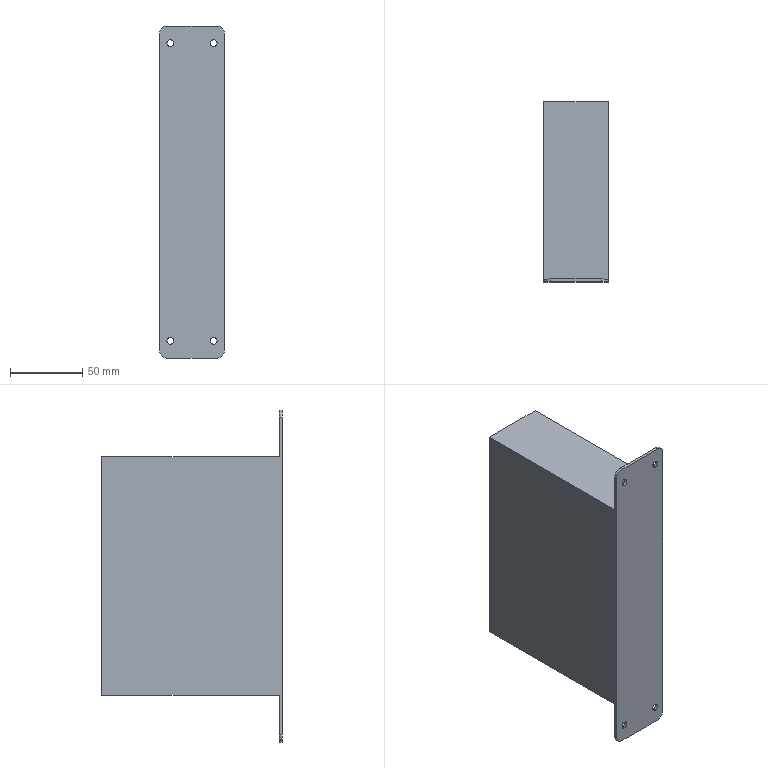Part | SolidWorks | features Extrusion 1, Fillet 1, HoleWzd 1, ICE 1 | 1 solid | 22 faces | box 45 x 125 x 230 mm | volume 933787 mm3 | cylinder 12 | plane 10 | commonest cylinder face diameters 4.8 x8 10 x4
STEP:
#1=CARTESIAN_POINT('',(-15.,0.,-105.4));
#2=VERTEX_POINT('',#1);
#3=CARTESIAN_POINT('',(-15.,0.,-100.6));
#4=VERTEX_POINT('',#3);
#5=CARTESIAN_POINT('',(-15.,0.,-103.));
#6=DIRECTION('',(0.,1.,0.));
#7=DIRECTION('',(0.,0.,1.));
#8=AXIS2_PLACEMENT_3D('',#5,#6,#7);
#9=CIRCLE('',#8,2.4);
#10=EDGE_CURVE('',#2,#4,#9,.T.);
#11=ORIENTED_EDGE('',*,*,#10,.F.);
#12=CARTESIAN_POINT('',(-15.,2.,-105.4));
#13=VERTEX_POINT('',#12);
#14=CARTESIAN_POINT('',(-15.,2.,-105.4));
#15=DIRECTION('',(0.,1.,0.));
#16=VECTOR('',#15,1000.);
#17=LINE('',#14,#16);
#18=EDGE_CURVE('',#2,#13,#17,.T.);
#19=ORIENTED_EDGE('',*,*,#18,.T.);
#20=CARTESIAN_POINT('',(-15.,2.,-100.6));
#21=VERTEX_POINT('',#20);
#22=CARTESIAN_POINT('',(-15.,2.,-103.));
#23=DIRECTION('',(0.,1.,0.));
#24=DIRECTION('',(0.,0.,1.));
#25=AXIS2_PLACEMENT_3D('',#22,#23,#24);
#26=CIRCLE('',#25,2.4);
#27=EDGE_CURVE('',#13,#21,#26,.T.);
#28=ORIENTED_EDGE('',*,*,#27,.T.);
#29=CARTESIAN_POINT('',(-15.,2.,-100.6));
#30=DIRECTION('',(0.,1.,0.));
#31=VECTOR('',#30,1000.);
#32=LINE('',#29,#31);
#33=EDGE_CURVE('',#4,#21,#32,.T.);
#34=ORIENTED_EDGE('',*,*,#33,.F.);
#35=EDGE_LOOP('',(#11,#19,#28,#34));
#36=FACE_OUTER_BOUND('',#35,.T.);
#37=CARTESIAN_POINT('',(-15.,2.,-103.));
#38=DIRECTION('',(0.,1.,0.));
#39=DIRECTION('',(0.,0.,1.));
#40=AXIS2_PLACEMENT_3D('',#37,#38,#39);
#41=CYLINDRICAL_SURFACE('',#40,2.4);
#42=ADVANCED_FACE('',(#36),#41,.F.);
#43=CARTESIAN_POINT('',(15.,0.,-105.4));
#44=VERTEX_POINT('',#43);
#45=CARTESIAN_POINT('',(15.,0.,-100.6));
#46=VERTEX_POINT('',#45);
#47=CARTESIAN_POINT('',(15.,0.,-103.));
#48=DIRECTION('',(0.,1.,0.));
#49=DIRECTION('',(0.,0.,1.));
#50=AXIS2_PLACEMENT_3D('',#47,#48,#49);
#51=CIRCLE('',#50,2.4);
#52=EDGE_CURVE('',#44,#46,#51,.T.);
#53=ORIENTED_EDGE('',*,*,#52,.F.);
#54=CARTESIAN_POINT('',(15.,2.,-105.4));
#55=VERTEX_POINT('',#54);
#56=CARTESIAN_POINT('',(15.,2.,-105.4));
#57=DIRECTION('',(0.,1.,0.));
#58=VECTOR('',#57,1000.);
#59=LINE('',#56,#58);
#60=EDGE_CURVE('',#44,#55,#59,.T.);
#61=ORIENTED_EDGE('',*,*,#60,.T.);
#62=CARTESIAN_POINT('',(15.,2.,-100.6));
#63=VERTEX_POINT('',#62);
#64=CARTESIAN_POINT('',(15.,2.,-103.));
#65=DIRECTION('',(0.,1.,0.));
#66=DIRECTION('',(0.,0.,1.));
#67=AXIS2_PLACEMENT_3D('',#64,#65,#66);
#68=CIRCLE('',#67,2.4);
#69=EDGE_CURVE('',#55,#63,#68,.T.);
#70=ORIENTED_EDGE('',*,*,#69,.T.);
#71=CARTESIAN_POINT('',(15.,2.,-100.6));
#72=DIRECTION('',(0.,1.,0.));
#73=VECTOR('',#72,1000.);
#74=LINE('',#71,#73);
#75=EDGE_CURVE('',#46,#63,#74,.T.);
#76=ORIENTED_EDGE('',*,*,#75,.F.);
#77=EDGE_LOOP('',(#53,#61,#70,#76));
#78=FACE_OUTER_BOUND('',#77,.T.);
#79=CARTESIAN_POINT('',(15.,2.,-103.));
#80=DIRECTION('',(0.,1.,0.));
#81=DIRECTION('',(0.,0.,1.));
#82=AXIS2_PLACEMENT_3D('',#79,#80,#81);
#83=CYLINDRICAL_SURFACE('',#82,2.4);
#84=ADVANCED_FACE('',(#78),#83,.F.);
#85=CARTESIAN_POINT('',(15.,0.,100.6));
#86=VERTEX_POINT('',#85);
#87=CARTESIAN_POINT('',(15.,0.,105.4));
#88=VERTEX_POINT('',#87);
#89=CARTESIAN_POINT('',(15.,0.,103.));
#90=DIRECTION('',(0.,1.,0.));
#91=DIRECTION('',(0.,0.,1.));
#92=AXIS2_PLACEMENT_3D('',#89,#90,#91);
#93=CIRCLE('',#92,2.4);
#94=EDGE_CURVE('',#86,#88,#93,.T.);
#95=ORIENTED_EDGE('',*,*,#94,.F.);
#96=CARTESIAN_POINT('',(15.,2.,100.6));
#97=VERTEX_POINT('',#96);
#98=CARTESIAN_POINT('',(15.,2.,100.6));
#99=DIRECTION('',(0.,1.,0.));
#100=VECTOR('',#99,1000.);
#101=LINE('',#98,#100);
#102=EDGE_CURVE('',#86,#97,#101,.T.);
#103=ORIENTED_EDGE('',*,*,#102,.T.);
#104=CARTESIAN_POINT('',(15.,2.,105.4));
#105=VERTEX_POINT('',#104);
#106=CARTESIAN_POINT('',(15.,2.,103.));
#107=DIRECTION('',(0.,1.,0.));
#108=DIRECTION('',(0.,0.,1.));
#109=AXIS2_PLACEMENT_3D('',#106,#107,#108);
#110=CIRCLE('',#109,2.4);
#111=EDGE_CURVE('',#97,#105,#110,.T.);
#112=ORIENTED_EDGE('',*,*,#111,.T.);
#113=CARTESIAN_POINT('',(15.,2.,105.4));
#114=DIRECTION('',(0.,1.,0.));
#115=VECTOR('',#114,1000.);
#116=LINE('',#113,#115);
#117=EDGE_CURVE('',#88,#105,#116,.T.);
#118=ORIENTED_EDGE('',*,*,#117,.F.);
#119=EDGE_LOOP('',(#95,#103,#112,#118));
#120=FACE_OUTER_BOUND('',#119,.T.);
#121=CARTESIAN_POINT('',(15.,2.,103.));
#122=DIRECTION('',(0.,1.,0.));
#123=DIRECTION('',(0.,0.,1.));
#124=AXIS2_PLACEMENT_3D('',#121,#122,#123);
#125=CYLINDRICAL_SURFACE('',#124,2.4);
#126=ADVANCED_FACE('',(#120),#125,.F.);
#127=CARTESIAN_POINT('',(-15.,0.,100.6));
#128=VERTEX_POINT('',#127);
#129=CARTESIAN_POINT('',(-15.,0.,105.4));
#130=VERTEX_POINT('',#129);
#131=CARTESIAN_POINT('',(-15.,0.,103.));
#132=DIRECTION('',(0.,1.,0.));
#133=DIRECTION('',(0.,0.,1.));
#134=AXIS2_PLACEMENT_3D('',#131,#132,#133);
#135=CIRCLE('',#134,2.4);
#136=EDGE_CURVE('',#128,#130,#135,.T.);
#137=ORIENTED_EDGE('',*,*,#136,.F.);
#138=CARTESIAN_POINT('',(-15.,2.,100.6));
#139=VERTEX_POINT('',#138);
#140=CARTESIAN_POINT('',(-15.,2.,100.6));
#141=DIRECTION('',(0.,1.,0.));
#142=VECTOR('',#141,1000.);
#143=LINE('',#140,#142);
#144=EDGE_CURVE('',#128,#139,#143,.T.);
#145=ORIENTED_EDGE('',*,*,#144,.T.);
#146=CARTESIAN_POINT('',(-15.,2.,105.4));
#147=VERTEX_POINT('',#146);
#148=CARTESIAN_POINT('',(-15.,2.,103.));
#149=DIRECTION('',(0.,1.,0.));
#150=DIRECTION('',(0.,0.,1.));
#151=AXIS2_PLACEMENT_3D('',#148,#149,#150);
#152=CIRCLE('',#151,2.4);
#153=EDGE_CURVE('',#139,#147,#152,.T.);
#154=ORIENTED_EDGE('',*,*,#153,.T.);
#155=CARTESIAN_POINT('',(-15.,2.,105.4));
#156=DIRECTION('',(0.,1.,0.));
#157=VECTOR('',#156,1000.);
#158=LINE('',#155,#157);
#159=EDGE_CURVE('',#130,#147,#158,.T.);
#160=ORIENTED_EDGE('',*,*,#159,.F.);
#161=EDGE_LOOP('',(#137,#145,#154,#160));
#162=FACE_OUTER_BOUND('',#161,.T.);
#163=CARTESIAN_POINT('',(-15.,2.,103.));
#164=DIRECTION('',(0.,1.,0.));
#165=DIRECTION('',(0.,0.,1.));
#166=AXIS2_PLACEMENT_3D('',#163,#164,#165);
#167=CYLINDRICAL_SURFACE('',#166,2.4);
#168=ADVANCED_FACE('',(#162),#167,.F.);
#169=CARTESIAN_POINT('',(22.5,2.,82.5));
#170=VERTEX_POINT('',#169);
#171=CARTESIAN_POINT('',(-22.5,2.,82.5));
#172=VERTEX_POINT('',#171);
#173=CARTESIAN_POINT('',(-22.5,2.,82.5));
#174=DIRECTION('',(-1.,0.,0.));
#175=VECTOR('',#174,1000.);
#176=LINE('',#173,#175);
#177=EDGE_CURVE('',#170,#172,#176,.T.);
#178=ORIENTED_EDGE('',*,*,#177,.F.);
#179=CARTESIAN_POINT('',(22.5,125.,82.5));
#180=VERTEX_POINT('',#179);
#181=CARTESIAN_POINT('',(22.5,125.,82.5));
#182=DIRECTION('',(0.,-1.,0.));
#183=VECTOR('',#182,1000.);
#184=LINE('',#181,#183);
#185=EDGE_CURVE('',#180,#170,#184,.T.);
#186=ORIENTED_EDGE('',*,*,#185,.F.);
#187=CARTESIAN_POINT('',(-22.5,125.,82.5));
#188=VERTEX_POINT('',#187);
#189=CARTESIAN_POINT('',(-22.5,125.,82.5));
#190=DIRECTION('',(1.,0.,0.));
#191=VECTOR('',#190,1000.);
#192=LINE('',#189,#191);
#193=EDGE_CURVE('',#188,#180,#192,.T.);
#194=ORIENTED_EDGE('',*,*,#193,.F.);
#195=CARTESIAN_POINT('',(-22.5,125.,82.5));
#196=DIRECTION('',(0.,-1.,0.));
#197=VECTOR('',#196,1000.);
#198=LINE('',#195,#197);
#199=EDGE_CURVE('',#188,#172,#198,.T.);
#200=ORIENTED_EDGE('',*,*,#199,.T.);
#201=EDGE_LOOP('',(#178,#186,#194,#200));
#202=FACE_OUTER_BOUND('',#201,.T.);
#203=CARTESIAN_POINT('',(-22.5,125.,82.5));
#204=DIRECTION('',(0.,0.,-1.));
#205=DIRECTION('',(-1.,0.,0.));
#206=AXIS2_PLACEMENT_3D('',#203,#204,#205);
#207=PLANE('',#206);
#208=ADVANCED_FACE('',(#202),#207,.F.);
#209=CARTESIAN_POINT('',(-22.5,2.,-82.5));
#210=VERTEX_POINT('',#209);
#211=CARTESIAN_POINT('',(22.5,2.,-82.5));
#212=VERTEX_POINT('',#211);
#213=CARTESIAN_POINT('',(-22.5,2.,-82.5));
#214=DIRECTION('',(1.,0.,0.));
#215=VECTOR('',#214,1000.);
#216=LINE('',#213,#215);
#217=EDGE_CURVE('',#210,#212,#216,.T.);
#218=ORIENTED_EDGE('',*,*,#217,.F.);
#219=CARTESIAN_POINT('',(-22.5,125.,-82.5));
#220=VERTEX_POINT('',#219);
#221=CARTESIAN_POINT('',(-22.5,125.,-82.5));
#222=DIRECTION('',(0.,-1.,0.));
#223=VECTOR('',#222,1000.);
#224=LINE('',#221,#223);
#225=EDGE_CURVE('',#220,#210,#224,.T.);
#226=ORIENTED_EDGE('',*,*,#225,.F.);
#227=CARTESIAN_POINT('',(22.5,125.,-82.5));
#228=VERTEX_POINT('',#227);
#229=CARTESIAN_POINT('',(-22.5,125.,-82.5));
#230=DIRECTION('',(-1.,0.,0.));
#231=VECTOR('',#230,1000.);
#232=LINE('',#229,#231);
#233=EDGE_CURVE('',#228,#220,#232,.T.);
#234=ORIENTED_EDGE('',*,*,#233,.F.);
#235=CARTESIAN_POINT('',(22.5,125.,-82.5));
#236=DIRECTION('',(0.,-1.,0.));
#237=VECTOR('',#236,1000.);
#238=LINE('',#235,#237);
#239=EDGE_CURVE('',#228,#212,#238,.T.);
#240=ORIENTED_EDGE('',*,*,#239,.T.);
#241=EDGE_LOOP('',(#218,#226,#234,#240));
#242=FACE_OUTER_BOUND('',#241,.T.);
#243=CARTESIAN_POINT('',(-22.5,125.,-82.5));
#244=DIRECTION('',(0.,0.,1.));
#245=DIRECTION('',(1.,0.,0.));
#246=AXIS2_PLACEMENT_3D('',#243,#244,#245);
#247=PLANE('',#246);
#248=ADVANCED_FACE('',(#242),#247,.F.);
#249=CARTESIAN_POINT('',(22.5,2.,110.));
#250=VERTEX_POINT('',#249);
#251=CARTESIAN_POINT('',(22.5,2.,82.5));
#252=DIRECTION('',(0.,0.,-1.));
#253=VECTOR('',#252,1000.);
#254=LINE('',#251,#253);
#255=EDGE_CURVE('',#250,#170,#254,.T.);
#256=ORIENTED_EDGE('',*,*,#255,.F.);
#257=CARTESIAN_POINT('',(22.5,0.,110.));
#258=VERTEX_POINT('',#257);
#259=CARTESIAN_POINT('',(22.5,125.,110.));
#260=DIRECTION('',(0.,-1.,0.));
#261=VECTOR('',#260,1000.);
#262=LINE('',#259,#261);
#263=EDGE_CURVE('',#250,#258,#262,.T.);
#264=ORIENTED_EDGE('',*,*,#263,.T.);
#265=CARTESIAN_POINT('',(22.5,0.,-110.));
#266=VERTEX_POINT('',#265);
#267=CARTESIAN_POINT('',(22.5,0.,82.5));
#268=DIRECTION('',(0.,0.,-1.));
#269=VECTOR('',#268,1000.);
#270=LINE('',#267,#269);
#271=EDGE_CURVE('',#258,#266,#270,.T.);
#272=ORIENTED_EDGE('',*,*,#271,.T.);
#273=CARTESIAN_POINT('',(22.5,2.,-110.));
#274=VERTEX_POINT('',#273);
#275=CARTESIAN_POINT('',(22.5,125.,-110.));
#276=DIRECTION('',(0.,1.,0.));
#277=VECTOR('',#276,1000.);
#278=LINE('',#275,#277);
#279=EDGE_CURVE('',#266,#274,#278,.T.);
#280=ORIENTED_EDGE('',*,*,#279,.T.);
#281=CARTESIAN_POINT('',(22.5,2.,-82.5));
#282=DIRECTION('',(0.,0.,-1.));
#283=VECTOR('',#282,1000.);
#284=LINE('',#281,#283);
#285=EDGE_CURVE('',#212,#274,#284,.T.);
#286=ORIENTED_EDGE('',*,*,#285,.F.);
#287=ORIENTED_EDGE('',*,*,#239,.F.);
#288=CARTESIAN_POINT('',(22.5,125.,82.5));
#289=DIRECTION('',(0.,0.,-1.));
#290=VECTOR('',#289,1000.);
#291=LINE('',#288,#290);
#292=EDGE_CURVE('',#180,#228,#291,.T.);
#293=ORIENTED_EDGE('',*,*,#292,.F.);
#294=ORIENTED_EDGE('',*,*,#185,.T.);
#295=EDGE_LOOP('',(#256,#264,#272,#280,#286,#287,#293,#294));
#296=FACE_OUTER_BOUND('',#295,.T.);
#297=CARTESIAN_POINT('',(22.5,125.,82.5));
#298=DIRECTION('',(-1.,0.,0.));
#299=DIRECTION('',(0.,0.,1.));
#300=AXIS2_PLACEMENT_3D('',#297,#298,#299);
#301=PLANE('',#300);
#302=ADVANCED_FACE('',(#296),#301,.F.);
#303=CARTESIAN_POINT('',(-22.5,0.,-110.));
#304=VERTEX_POINT('',#303);
#305=CARTESIAN_POINT('',(-22.5,0.,110.));
#306=VERTEX_POINT('',#305);
#307=CARTESIAN_POINT('',(-22.5,0.,82.5));
#308=DIRECTION('',(0.,0.,1.));
#309=VECTOR('',#308,1000.);
#310=LINE('',#307,#309);
#311=EDGE_CURVE('',#304,#306,#310,.T.);
#312=ORIENTED_EDGE('',*,*,#311,.T.);
#313=CARTESIAN_POINT('',(-22.5,2.,110.));
#314=VERTEX_POINT('',#313);
#315=CARTESIAN_POINT('',(-22.5,125.,110.));
#316=DIRECTION('',(0.,1.,0.));
#317=VECTOR('',#316,1000.);
#318=LINE('',#315,#317);
#319=EDGE_CURVE('',#306,#314,#318,.T.);
#320=ORIENTED_EDGE('',*,*,#319,.T.);
#321=CARTESIAN_POINT('',(-22.5,2.,82.5));
#322=DIRECTION('',(0.,0.,1.));
#323=VECTOR('',#322,1000.);
#324=LINE('',#321,#323);
#325=EDGE_CURVE('',#172,#314,#324,.T.);
#326=ORIENTED_EDGE('',*,*,#325,.F.);
#327=ORIENTED_EDGE('',*,*,#199,.F.);
#328=CARTESIAN_POINT('',(-22.5,125.,82.5));
#329=DIRECTION('',(0.,0.,1.));
#330=VECTOR('',#329,1000.);
#331=LINE('',#328,#330);
#332=EDGE_CURVE('',#220,#188,#331,.T.);
#333=ORIENTED_EDGE('',*,*,#332,.F.);
#334=ORIENTED_EDGE('',*,*,#225,.T.);
#335=CARTESIAN_POINT('',(-22.5,2.,-110.));
#336=VERTEX_POINT('',#335);
#337=CARTESIAN_POINT('',(-22.5,2.,-82.5));
#338=DIRECTION('',(0.,0.,1.));
#339=VECTOR('',#338,1000.);
#340=LINE('',#337,#339);
#341=EDGE_CURVE('',#336,#210,#340,.T.);
#342=ORIENTED_EDGE('',*,*,#341,.F.);
#343=CARTESIAN_POINT('',(-22.5,125.,-110.));
#344=DIRECTION('',(0.,-1.,0.));
#345=VECTOR('',#344,1000.);
#346=LINE('',#343,#345);
#347=EDGE_CURVE('',#336,#304,#346,.T.);
#348=ORIENTED_EDGE('',*,*,#347,.T.);
#349=EDGE_LOOP('',(#312,#320,#326,#327,#333,#334,#342,#348));
#350=FACE_OUTER_BOUND('',#349,.T.);
#351=CARTESIAN_POINT('',(-22.5,125.,82.5));
#352=DIRECTION('',(1.,0.,0.));
#353=DIRECTION('',(0.,0.,-1.));
#354=AXIS2_PLACEMENT_3D('',#351,#352,#353);
#355=PLANE('',#354);
#356=ADVANCED_FACE('',(#350),#355,.F.);
#357=ORIENTED_EDGE('',*,*,#292,.T.);
#358=ORIENTED_EDGE('',*,*,#233,.T.);
#359=ORIENTED_EDGE('',*,*,#332,.T.);
#360=ORIENTED_EDGE('',*,*,#193,.T.);
#361=EDGE_LOOP('',(#357,#358,#359,#360));
#362=FACE_OUTER_BOUND('',#361,.T.);
#363=CARTESIAN_POINT('',(0.,125.,0.));
#364=DIRECTION('',(0.,-1.,0.));
#365=DIRECTION('',(0.,0.,-1.));
#366=AXIS2_PLACEMENT_3D('',#363,#364,#365);
#367=PLANE('',#366);
#368=ADVANCED_FACE('',(#362),#367,.F.);
#369=CARTESIAN_POINT('',(-15.,0.,-103.));
#370=DIRECTION('',(0.,1.,0.));
#371=DIRECTION('',(0.,0.,1.));
#372=AXIS2_PLACEMENT_3D('',#369,#370,#371);
#373=CIRCLE('',#372,2.4);
#374=EDGE_CURVE('',#4,#2,#373,.T.);
#375=ORIENTED_EDGE('',*,*,#374,.T.);
#376=ORIENTED_EDGE('',*,*,#10,.T.);
#377=EDGE_LOOP('',(#375,#376));
#378=FACE_BOUND('',#377,.T.);
#379=CARTESIAN_POINT('',(15.,0.,-103.));
#380=DIRECTION('',(0.,1.,0.));
#381=DIRECTION('',(0.,0.,1.));
#382=AXIS2_PLACEMENT_3D('',#379,#380,#381);
#383=CIRCLE('',#382,2.4);
#384=EDGE_CURVE('',#46,#44,#383,.T.);
#385=ORIENTED_EDGE('',*,*,#384,.T.);
#386=ORIENTED_EDGE('',*,*,#52,.T.);
#387=EDGE_LOOP('',(#385,#386));
#388=FACE_BOUND('',#387,.T.);
#389=CARTESIAN_POINT('',(15.,0.,103.));
#390=DIRECTION('',(0.,1.,0.));
#391=DIRECTION('',(0.,0.,1.));
#392=AXIS2_PLACEMENT_3D('',#389,#390,#391);
#393=CIRCLE('',#392,2.4);
#394=EDGE_CURVE('',#88,#86,#393,.T.);
#395=ORIENTED_EDGE('',*,*,#394,.T.);
#396=ORIENTED_EDGE('',*,*,#94,.T.);
#397=EDGE_LOOP('',(#395,#396));
#398=FACE_BOUND('',#397,.T.);
#399=CARTESIAN_POINT('',(-15.,0.,103.));
#400=DIRECTION('',(0.,1.,0.));
#401=DIRECTION('',(0.,0.,1.));
#402=AXIS2_PLACEMENT_3D('',#399,#400,#401);
#403=CIRCLE('',#402,2.4);
#404=EDGE_CURVE('',#130,#128,#403,.T.);
#405=ORIENTED_EDGE('',*,*,#404,.T.);
#406=ORIENTED_EDGE('',*,*,#136,.T.);
#407=EDGE_LOOP('',(#405,#406));
#408=FACE_BOUND('',#407,.T.);
#409=CARTESIAN_POINT('',(-17.5,0.,115.));
#410=VERTEX_POINT('',#409);
#411=CARTESIAN_POINT('',(17.5,0.,115.));
#412=VERTEX_POINT('',#411);
#413=CARTESIAN_POINT('',(-22.5,0.,115.));
#414=DIRECTION('',(1.,0.,0.));
#415=VECTOR('',#414,1000.);
#416=LINE('',#413,#415);
#417=EDGE_CURVE('',#410,#412,#416,.T.);
#418=ORIENTED_EDGE('',*,*,#417,.F.);
#419=CARTESIAN_POINT('',(-17.5,0.,110.));
#420=DIRECTION('',(0.,-1.,0.));
#421=DIRECTION('',(0.,0.,-1.));
#422=AXIS2_PLACEMENT_3D('',#419,#420,#421);
#423=CIRCLE('',#422,5.);
#424=EDGE_CURVE('',#410,#306,#423,.T.);
#425=ORIENTED_EDGE('',*,*,#424,.T.);
#426=ORIENTED_EDGE('',*,*,#311,.F.);
#427=CARTESIAN_POINT('',(-17.5,0.,-115.));
#428=VERTEX_POINT('',#427);
#429=CARTESIAN_POINT('',(-17.5,0.,-110.));
#430=DIRECTION('',(0.,-1.,0.));
#431=DIRECTION('',(0.,0.,-1.));
#432=AXIS2_PLACEMENT_3D('',#429,#430,#431);
#433=CIRCLE('',#432,5.);
#434=EDGE_CURVE('',#304,#428,#433,.T.);
#435=ORIENTED_EDGE('',*,*,#434,.T.);
#436=CARTESIAN_POINT('',(17.5,0.,-115.));
#437=VERTEX_POINT('',#436);
#438=CARTESIAN_POINT('',(-22.5,0.,-115.));
#439=DIRECTION('',(-1.,0.,0.));
#440=VECTOR('',#439,1000.);
#441=LINE('',#438,#440);
#442=EDGE_CURVE('',#437,#428,#441,.T.);
#443=ORIENTED_EDGE('',*,*,#442,.F.);
#444=CARTESIAN_POINT('',(17.5,0.,-110.));
#445=DIRECTION('',(0.,-1.,0.));
#446=DIRECTION('',(0.,0.,-1.));
#447=AXIS2_PLACEMENT_3D('',#444,#445,#446);
#448=CIRCLE('',#447,5.);
#449=EDGE_CURVE('',#437,#266,#448,.T.);
#450=ORIENTED_EDGE('',*,*,#449,.T.);
#451=ORIENTED_EDGE('',*,*,#271,.F.);
#452=CARTESIAN_POINT('',(17.5,0.,110.));
#453=DIRECTION('',(0.,-1.,0.));
#454=DIRECTION('',(0.,0.,-1.));
#455=AXIS2_PLACEMENT_3D('',#452,#453,#454);
#456=CIRCLE('',#455,5.);
#457=EDGE_CURVE('',#258,#412,#456,.T.);
#458=ORIENTED_EDGE('',*,*,#457,.T.);
#459=EDGE_LOOP('',(#418,#425,#426,#435,#443,#450,#451,#458));
#460=FACE_OUTER_BOUND('',#459,.T.);
#461=CARTESIAN_POINT('',(0.,0.,0.));
#462=DIRECTION('',(0.,-1.,0.));
#463=DIRECTION('',(0.,0.,-1.));
#464=AXIS2_PLACEMENT_3D('',#461,#462,#463);
#465=PLANE('',#464);
#466=ADVANCED_FACE('',(#378,#388,#398,#408,#460),#465,.T.);
#467=CARTESIAN_POINT('',(17.5,2.,-115.));
#468=VERTEX_POINT('',#467);
#469=CARTESIAN_POINT('',(-17.5,2.,-115.));
#470=VERTEX_POINT('',#469);
#471=CARTESIAN_POINT('',(-22.5,2.,-115.));
#472=DIRECTION('',(-1.,0.,0.));
#473=VECTOR('',#472,1000.);
#474=LINE('',#471,#473);
#475=EDGE_CURVE('',#468,#470,#474,.T.);
#476=ORIENTED_EDGE('',*,*,#475,.F.);
#477=CARTESIAN_POINT('',(17.5,2.,-115.));
#478=DIRECTION('',(0.,-1.,0.));
#479=VECTOR('',#478,1000.);
#480=LINE('',#477,#479);
#481=EDGE_CURVE('',#468,#437,#480,.T.);
#482=ORIENTED_EDGE('',*,*,#481,.T.);
#483=ORIENTED_EDGE('',*,*,#442,.T.);
#484=CARTESIAN_POINT('',(-17.5,2.,-115.));
#485=DIRECTION('',(0.,1.,0.));
#486=VECTOR('',#485,1000.);
#487=LINE('',#484,#486);
#488=EDGE_CURVE('',#428,#470,#487,.T.);
#489=ORIENTED_EDGE('',*,*,#488,.T.);
#490=EDGE_LOOP('',(#476,#482,#483,#489));
#491=FACE_OUTER_BOUND('',#490,.T.);
#492=CARTESIAN_POINT('',(-22.5,2.,-115.));
#493=DIRECTION('',(0.,0.,1.));
#494=DIRECTION('',(1.,0.,0.));
#495=AXIS2_PLACEMENT_3D('',#492,#493,#494);
#496=PLANE('',#495);
#497=ADVANCED_FACE('',(#491),#496,.F.);
#498=CARTESIAN_POINT('',(-15.,2.,-103.));
#499=DIRECTION('',(0.,1.,0.));
#500=DIRECTION('',(0.,0.,1.));
#501=AXIS2_PLACEMENT_3D('',#498,#499,#500);
#502=CIRCLE('',#501,2.4);
#503=EDGE_CURVE('',#21,#13,#502,.T.);
#504=ORIENTED_EDGE('',*,*,#503,.F.);
#505=ORIENTED_EDGE('',*,*,#27,.F.);
#506=EDGE_LOOP('',(#504,#505));
#507=FACE_BOUND('',#506,.T.);
#508=CARTESIAN_POINT('',(15.,2.,-103.));
#509=DIRECTION('',(0.,1.,0.));
#510=DIRECTION('',(0.,0.,1.));
#511=AXIS2_PLACEMENT_3D('',#508,#509,#510);
#512=CIRCLE('',#511,2.4);
#513=EDGE_CURVE('',#63,#55,#512,.T.);
#514=ORIENTED_EDGE('',*,*,#513,.F.);
#515=ORIENTED_EDGE('',*,*,#69,.F.);
#516=EDGE_LOOP('',(#514,#515));
#517=FACE_BOUND('',#516,.T.);
#518=ORIENTED_EDGE('',*,*,#285,.T.);
#519=CARTESIAN_POINT('',(17.5,2.,-110.));
#520=DIRECTION('',(0.,1.,0.));
#521=DIRECTION('',(0.,0.,-1.));
#522=AXIS2_PLACEMENT_3D('',#519,#520,#521);
#523=CIRCLE('',#522,5.);
#524=EDGE_CURVE('',#274,#468,#523,.T.);
#525=ORIENTED_EDGE('',*,*,#524,.T.);
#526=ORIENTED_EDGE('',*,*,#475,.T.);
#527=CARTESIAN_POINT('',(-17.5,2.,-110.));
#528=DIRECTION('',(0.,1.,0.));
#529=DIRECTION('',(0.,0.,-1.));
#530=AXIS2_PLACEMENT_3D('',#527,#528,#529);
#531=CIRCLE('',#530,5.);
#532=EDGE_CURVE('',#470,#336,#531,.T.);
#533=ORIENTED_EDGE('',*,*,#532,.T.);
#534=ORIENTED_EDGE('',*,*,#341,.T.);
#535=ORIENTED_EDGE('',*,*,#217,.T.);
#536=EDGE_LOOP('',(#518,#525,#526,#533,#534,#535));
#537=FACE_OUTER_BOUND('',#536,.T.);
#538=CARTESIAN_POINT('',(0.,2.,0.));
#539=DIRECTION('',(0.,-1.,0.));
#540=DIRECTION('',(0.,0.,-1.));
#541=AXIS2_PLACEMENT_3D('',#538,#539,#540);
#542=PLANE('',#541);
#543=ADVANCED_FACE('',(#507,#517,#537),#542,.F.);
#544=CARTESIAN_POINT('',(-17.5,2.,115.));
#545=VERTEX_POINT('',#544);
#546=CARTESIAN_POINT('',(17.5,2.,115.));
#547=VERTEX_POINT('',#546);
#548=CARTESIAN_POINT('',(-22.5,2.,115.));
#549=DIRECTION('',(1.,0.,0.));
#550=VECTOR('',#549,1000.);
#551=LINE('',#548,#550);
#552=EDGE_CURVE('',#545,#547,#551,.T.);
#553=ORIENTED_EDGE('',*,*,#552,.F.);
#554=CARTESIAN_POINT('',(-17.5,2.,115.));
#555=DIRECTION('',(0.,-1.,0.));
#556=VECTOR('',#555,1000.);
#557=LINE('',#554,#556);
#558=EDGE_CURVE('',#545,#410,#557,.T.);
#559=ORIENTED_EDGE('',*,*,#558,.T.);
#560=ORIENTED_EDGE('',*,*,#417,.T.);
#561=CARTESIAN_POINT('',(17.5,2.,115.));
#562=DIRECTION('',(0.,1.,0.));
#563=VECTOR('',#562,1000.);
#564=LINE('',#561,#563);
#565=EDGE_CURVE('',#412,#547,#564,.T.);
#566=ORIENTED_EDGE('',*,*,#565,.T.);
#567=EDGE_LOOP('',(#553,#559,#560,#566));
#568=FACE_OUTER_BOUND('',#567,.T.);
#569=CARTESIAN_POINT('',(-22.5,2.,115.));
#570=DIRECTION('',(0.,0.,-1.));
#571=DIRECTION('',(-1.,0.,0.));
#572=AXIS2_PLACEMENT_3D('',#569,#570,#571);
#573=PLANE('',#572);
#574=ADVANCED_FACE('',(#568),#573,.F.);
#575=CARTESIAN_POINT('',(15.,2.,103.));
#576=DIRECTION('',(0.,1.,0.));
#577=DIRECTION('',(0.,0.,1.));
#578=AXIS2_PLACEMENT_3D('',#575,#576,#577);
#579=CIRCLE('',#578,2.4);
#580=EDGE_CURVE('',#105,#97,#579,.T.);
#581=ORIENTED_EDGE('',*,*,#580,.F.);
#582=ORIENTED_EDGE('',*,*,#111,.F.);
#583=EDGE_LOOP('',(#581,#582));
#584=FACE_BOUND('',#583,.T.);
#585=CARTESIAN_POINT('',(-15.,2.,103.));
#586=DIRECTION('',(0.,1.,0.));
#587=DIRECTION('',(0.,0.,1.));
#588=AXIS2_PLACEMENT_3D('',#585,#586,#587);
#589=CIRCLE('',#588,2.4);
#590=EDGE_CURVE('',#147,#139,#589,.T.);
#591=ORIENTED_EDGE('',*,*,#590,.F.);
#592=ORIENTED_EDGE('',*,*,#153,.F.);
#593=EDGE_LOOP('',(#591,#592));
#594=FACE_BOUND('',#593,.T.);
#595=ORIENTED_EDGE('',*,*,#325,.T.);
#596=CARTESIAN_POINT('',(-17.5,2.,110.));
#597=DIRECTION('',(0.,1.,0.));
#598=DIRECTION('',(0.,0.,-1.));
#599=AXIS2_PLACEMENT_3D('',#596,#597,#598);
#600=CIRCLE('',#599,5.);
#601=EDGE_CURVE('',#314,#545,#600,.T.);
#602=ORIENTED_EDGE('',*,*,#601,.T.);
#603=ORIENTED_EDGE('',*,*,#552,.T.);
#604=CARTESIAN_POINT('',(17.5,2.,110.));
#605=DIRECTION('',(0.,1.,0.));
#606=DIRECTION('',(0.,0.,-1.));
#607=AXIS2_PLACEMENT_3D('',#604,#605,#606);
#608=CIRCLE('',#607,5.);
#609=EDGE_CURVE('',#547,#250,#608,.T.);
#610=ORIENTED_EDGE('',*,*,#609,.T.);
#611=ORIENTED_EDGE('',*,*,#255,.T.);
#612=ORIENTED_EDGE('',*,*,#177,.T.);
#613=EDGE_LOOP('',(#595,#602,#603,#610,#611,#612));
#614=FACE_OUTER_BOUND('',#613,.T.);
#615=CARTESIAN_POINT('',(0.,2.,0.));
#616=DIRECTION('',(0.,-1.,0.));
#617=DIRECTION('',(0.,0.,-1.));
#618=AXIS2_PLACEMENT_3D('',#615,#616,#617);
#619=PLANE('',#618);
#620=ADVANCED_FACE('',(#584,#594,#614),#619,.F.);
#621=ORIENTED_EDGE('',*,*,#144,.F.);
#622=ORIENTED_EDGE('',*,*,#404,.F.);
#623=ORIENTED_EDGE('',*,*,#159,.T.);
#624=ORIENTED_EDGE('',*,*,#590,.T.);
#625=EDGE_LOOP('',(#621,#622,#623,#624));
#626=FACE_OUTER_BOUND('',#625,.T.);
#627=CARTESIAN_POINT('',(-15.,2.,103.));
#628=DIRECTION('',(0.,1.,0.));
#629=DIRECTION('',(0.,0.,1.));
#630=AXIS2_PLACEMENT_3D('',#627,#628,#629);
#631=CYLINDRICAL_SURFACE('',#630,2.4);
#632=ADVANCED_FACE('',(#626),#631,.F.);
#633=ORIENTED_EDGE('',*,*,#102,.F.);
#634=ORIENTED_EDGE('',*,*,#394,.F.);
#635=ORIENTED_EDGE('',*,*,#117,.T.);
#636=ORIENTED_EDGE('',*,*,#580,.T.);
#637=EDGE_LOOP('',(#633,#634,#635,#636));
#638=FACE_OUTER_BOUND('',#637,.T.);
#639=CARTESIAN_POINT('',(15.,2.,103.));
#640=DIRECTION('',(0.,1.,0.));
#641=DIRECTION('',(0.,0.,1.));
#642=AXIS2_PLACEMENT_3D('',#639,#640,#641);
#643=CYLINDRICAL_SURFACE('',#642,2.4);
#644=ADVANCED_FACE('',(#638),#643,.F.);
#645=ORIENTED_EDGE('',*,*,#60,.F.);
#646=ORIENTED_EDGE('',*,*,#384,.F.);
#647=ORIENTED_EDGE('',*,*,#75,.T.);
#648=ORIENTED_EDGE('',*,*,#513,.T.);
#649=EDGE_LOOP('',(#645,#646,#647,#648));
#650=FACE_OUTER_BOUND('',#649,.T.);
#651=CARTESIAN_POINT('',(15.,2.,-103.));
#652=DIRECTION('',(0.,1.,0.));
#653=DIRECTION('',(0.,0.,1.));
#654=AXIS2_PLACEMENT_3D('',#651,#652,#653);
#655=CYLINDRICAL_SURFACE('',#654,2.4);
#656=ADVANCED_FACE('',(#650),#655,.F.);
#657=ORIENTED_EDGE('',*,*,#18,.F.);
#658=ORIENTED_EDGE('',*,*,#374,.F.);
#659=ORIENTED_EDGE('',*,*,#33,.T.);
#660=ORIENTED_EDGE('',*,*,#503,.T.);
#661=EDGE_LOOP('',(#657,#658,#659,#660));
#662=FACE_OUTER_BOUND('',#661,.T.);
#663=CARTESIAN_POINT('',(-15.,2.,-103.));
#664=DIRECTION('',(0.,1.,0.));
#665=DIRECTION('',(0.,0.,1.));
#666=AXIS2_PLACEMENT_3D('',#663,#664,#665);
#667=CYLINDRICAL_SURFACE('',#666,2.4);
#668=ADVANCED_FACE('',(#662),#667,.F.);
#669=ORIENTED_EDGE('',*,*,#601,.F.);
#670=ORIENTED_EDGE('',*,*,#319,.F.);
#671=ORIENTED_EDGE('',*,*,#424,.F.);
#672=ORIENTED_EDGE('',*,*,#558,.F.);
#673=EDGE_LOOP('',(#669,#670,#671,#672));
#674=FACE_OUTER_BOUND('',#673,.T.);
#675=CARTESIAN_POINT('',(-17.5,2.,110.));
#676=DIRECTION('',(0.,-1.,0.));
#677=DIRECTION('',(0.,0.,-1.));
#678=AXIS2_PLACEMENT_3D('',#675,#676,#677);
#679=CYLINDRICAL_SURFACE('',#678,5.);
#680=ADVANCED_FACE('',(#674),#679,.T.);
#681=ORIENTED_EDGE('',*,*,#609,.F.);
#682=ORIENTED_EDGE('',*,*,#565,.F.);
#683=ORIENTED_EDGE('',*,*,#457,.F.);
#684=ORIENTED_EDGE('',*,*,#263,.F.);
#685=EDGE_LOOP('',(#681,#682,#683,#684));
#686=FACE_OUTER_BOUND('',#685,.T.);
#687=CARTESIAN_POINT('',(17.5,125.,110.));
#688=DIRECTION('',(0.,-1.,0.));
#689=DIRECTION('',(0.,0.,-1.));
#690=AXIS2_PLACEMENT_3D('',#687,#688,#689);
#691=CYLINDRICAL_SURFACE('',#690,5.);
#692=ADVANCED_FACE('',(#686),#691,.T.);
#693=ORIENTED_EDGE('',*,*,#524,.F.);
#694=ORIENTED_EDGE('',*,*,#279,.F.);
#695=ORIENTED_EDGE('',*,*,#449,.F.);
#696=ORIENTED_EDGE('',*,*,#481,.F.);
#697=EDGE_LOOP('',(#693,#694,#695,#696));
#698=FACE_OUTER_BOUND('',#697,.T.);
#699=CARTESIAN_POINT('',(17.5,2.,-110.));
#700=DIRECTION('',(0.,-1.,0.));
#701=DIRECTION('',(0.,0.,-1.));
#702=AXIS2_PLACEMENT_3D('',#699,#700,#701);
#703=CYLINDRICAL_SURFACE('',#702,5.);
#704=ADVANCED_FACE('',(#698),#703,.T.);
#705=ORIENTED_EDGE('',*,*,#532,.F.);
#706=ORIENTED_EDGE('',*,*,#488,.F.);
#707=ORIENTED_EDGE('',*,*,#434,.F.);
#708=ORIENTED_EDGE('',*,*,#347,.F.);
#709=EDGE_LOOP('',(#705,#706,#707,#708));
#710=FACE_OUTER_BOUND('',#709,.T.);
#711=CARTESIAN_POINT('',(-17.5,125.,-110.));
#712=DIRECTION('',(0.,-1.,0.));
#713=DIRECTION('',(0.,0.,-1.));
#714=AXIS2_PLACEMENT_3D('',#711,#712,#713);
#715=CYLINDRICAL_SURFACE('',#714,5.);
#716=ADVANCED_FACE('',(#710),#715,.T.);
#717=CLOSED_SHELL('',(#42,#84,#126,#168,#208,#248,#302,#356,#368,#466,#497,#543,#574,#620,#632,#644,#656,#668,#680,#692,#704,#716));
#718=MANIFOLD_SOLID_BREP('',#717);
#719=CARTESIAN_POINT('',(0.,0.,0.));
#720=DIRECTION('',(0.,0.,1.));
#721=DIRECTION('',(1.,0.,0.));
#722=AXIS2_PLACEMENT_3D('',#719,#720,#721);
#723=(LENGTH_UNIT()NAMED_UNIT(*)SI_UNIT(.MILLI.,.METRE.));
#724=UNCERTAINTY_MEASURE_WITH_UNIT(LENGTH_MEASURE(0.00001),#723,'','');
#725=(NAMED_UNIT(*)PLANE_ANGLE_UNIT()SI_UNIT($,.RADIAN.));
#726=(NAMED_UNIT(*)SI_UNIT($,.STERADIAN.)SOLID_ANGLE_UNIT());
#727=(GEOMETRIC_REPRESENTATION_CONTEXT(3)GLOBAL_UNCERTAINTY_ASSIGNED_CONTEXT((#724))GLOBAL_UNIT_ASSIGNED_CONTEXT((#723,#725,#726))REPRESENTATION_CONTEXT('',''));
#728=ADVANCED_BREP_SHAPE_REPRESENTATION('',(#718,#722),#727);